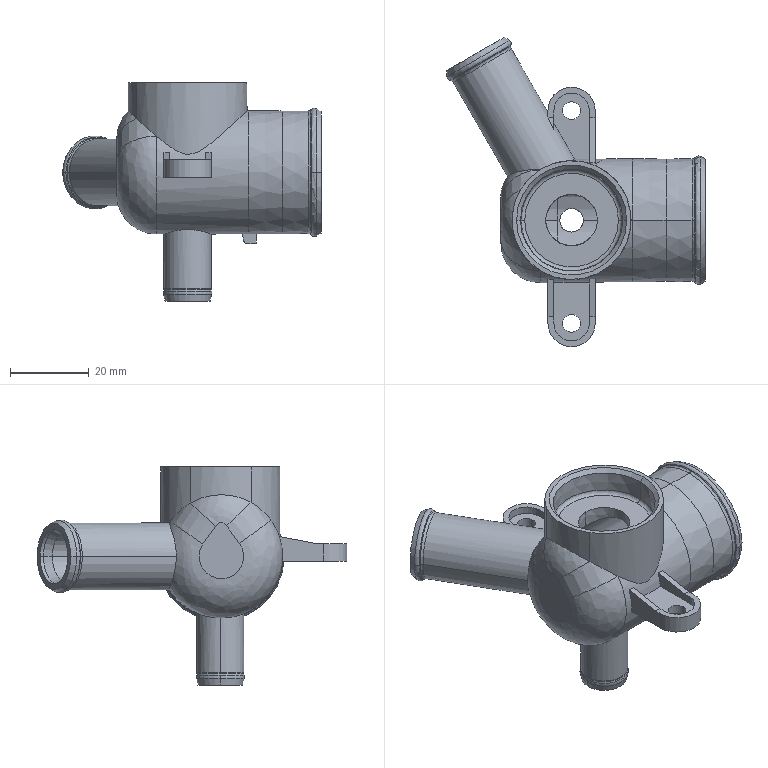Part | STEP file | ZXW722-L-39 | 1 solid | 112 faces | box 65.761 x 78.712 x 55.422 mm | volume 21689 mm3 | cylinder 34 | plane 30 | cone 28 | torus 14 | spline 6 | commonest cylinder face diameters 12 x6 4.5 x4 31.336 x4 6 x2 8 x2 9 x2